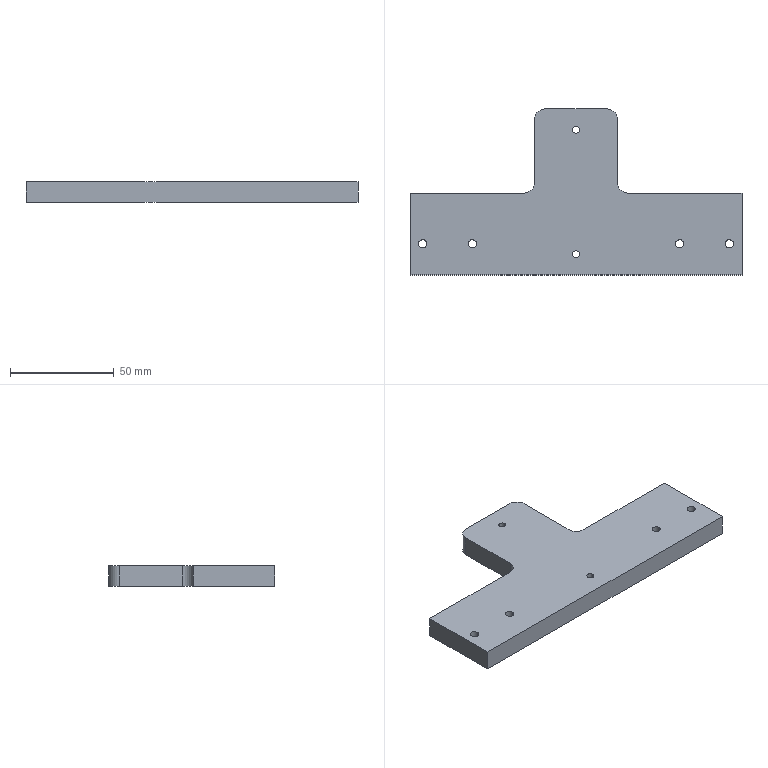Part | 1 solid | 26 faces | box 160 x 80 x 10 mm | volume 78726 mm3 | cylinder 16 | plane 10 | commonest cylinder face diameters 4 x8 3.3 x4 10 x4
STEP:
#1=CARTESIAN_POINT('',(1.65,-30.,0.));
#2=VERTEX_POINT('',#1);
#3=CARTESIAN_POINT('',(-1.65,-30.,0.));
#4=VERTEX_POINT('',#3);
#5=CARTESIAN_POINT('',(0.,-30.,0.));
#6=DIRECTION('',(0.,0.,-1.));
#7=DIRECTION('',(-1.,0.,0.));
#8=AXIS2_PLACEMENT_3D('',#5,#6,#7);
#9=CIRCLE('',#8,1.65);
#10=EDGE_CURVE('',#2,#4,#9,.T.);
#11=ORIENTED_EDGE('',*,*,#10,.T.);
#12=CARTESIAN_POINT('',(-1.65,-30.,10.));
#13=VERTEX_POINT('',#12);
#14=CARTESIAN_POINT('',(-1.65,-30.,10.));
#15=DIRECTION('',(0.,0.,1.));
#16=VECTOR('',#15,1000.);
#17=LINE('',#14,#16);
#18=EDGE_CURVE('',#4,#13,#17,.T.);
#19=ORIENTED_EDGE('',*,*,#18,.T.);
#20=CARTESIAN_POINT('',(1.65,-30.,10.));
#21=VERTEX_POINT('',#20);
#22=CARTESIAN_POINT('',(0.,-30.,10.));
#23=DIRECTION('',(0.,0.,1.));
#24=DIRECTION('',(1.,0.,0.));
#25=AXIS2_PLACEMENT_3D('',#22,#23,#24);
#26=CIRCLE('',#25,1.65);
#27=EDGE_CURVE('',#13,#21,#26,.T.);
#28=ORIENTED_EDGE('',*,*,#27,.T.);
#29=CARTESIAN_POINT('',(1.65,-30.,10.));
#30=DIRECTION('',(0.,0.,1.));
#31=VECTOR('',#30,1000.);
#32=LINE('',#29,#31);
#33=EDGE_CURVE('',#2,#21,#32,.T.);
#34=ORIENTED_EDGE('',*,*,#33,.F.);
#35=EDGE_LOOP('',(#11,#19,#28,#34));
#36=FACE_OUTER_BOUND('',#35,.T.);
#37=CARTESIAN_POINT('',(0.,-30.,10.));
#38=DIRECTION('',(0.,0.,1.));
#39=DIRECTION('',(1.,0.,0.));
#40=AXIS2_PLACEMENT_3D('',#37,#38,#39);
#41=CYLINDRICAL_SURFACE('',#40,1.65);
#42=ADVANCED_FACE('',(#36),#41,.F.);
#43=CARTESIAN_POINT('',(1.65,30.,0.));
#44=VERTEX_POINT('',#43);
#45=CARTESIAN_POINT('',(-1.65,30.,0.));
#46=VERTEX_POINT('',#45);
#47=CARTESIAN_POINT('',(0.,30.,0.));
#48=DIRECTION('',(0.,0.,-1.));
#49=DIRECTION('',(-1.,0.,0.));
#50=AXIS2_PLACEMENT_3D('',#47,#48,#49);
#51=CIRCLE('',#50,1.65);
#52=EDGE_CURVE('',#44,#46,#51,.T.);
#53=ORIENTED_EDGE('',*,*,#52,.T.);
#54=CARTESIAN_POINT('',(-1.65,30.,10.));
#55=VERTEX_POINT('',#54);
#56=CARTESIAN_POINT('',(-1.65,30.,10.));
#57=DIRECTION('',(0.,0.,1.));
#58=VECTOR('',#57,1000.);
#59=LINE('',#56,#58);
#60=EDGE_CURVE('',#46,#55,#59,.T.);
#61=ORIENTED_EDGE('',*,*,#60,.T.);
#62=CARTESIAN_POINT('',(1.65,30.,10.));
#63=VERTEX_POINT('',#62);
#64=CARTESIAN_POINT('',(0.,30.,10.));
#65=DIRECTION('',(0.,0.,1.));
#66=DIRECTION('',(1.,0.,0.));
#67=AXIS2_PLACEMENT_3D('',#64,#65,#66);
#68=CIRCLE('',#67,1.65);
#69=EDGE_CURVE('',#55,#63,#68,.T.);
#70=ORIENTED_EDGE('',*,*,#69,.T.);
#71=CARTESIAN_POINT('',(1.65,30.,10.));
#72=DIRECTION('',(0.,0.,1.));
#73=VECTOR('',#72,1000.);
#74=LINE('',#71,#73);
#75=EDGE_CURVE('',#44,#63,#74,.T.);
#76=ORIENTED_EDGE('',*,*,#75,.F.);
#77=EDGE_LOOP('',(#53,#61,#70,#76));
#78=FACE_OUTER_BOUND('',#77,.T.);
#79=CARTESIAN_POINT('',(0.,30.,10.));
#80=DIRECTION('',(0.,0.,1.));
#81=DIRECTION('',(1.,0.,0.));
#82=AXIS2_PLACEMENT_3D('',#79,#80,#81);
#83=CYLINDRICAL_SURFACE('',#82,1.65);
#84=ADVANCED_FACE('',(#78),#83,.F.);
#85=CARTESIAN_POINT('',(71.9,-25.,10.));
#86=VERTEX_POINT('',#85);
#87=CARTESIAN_POINT('',(75.9,-25.,10.));
#88=VERTEX_POINT('',#87);
#89=CARTESIAN_POINT('',(73.9,-25.,10.));
#90=DIRECTION('',(0.,0.,1.));
#91=DIRECTION('',(1.,0.,0.));
#92=AXIS2_PLACEMENT_3D('',#89,#90,#91);
#93=CIRCLE('',#92,2.);
#94=EDGE_CURVE('',#86,#88,#93,.T.);
#95=ORIENTED_EDGE('',*,*,#94,.T.);
#96=CARTESIAN_POINT('',(75.9,-25.,0.));
#97=VERTEX_POINT('',#96);
#98=CARTESIAN_POINT('',(75.9,-25.,10.));
#99=DIRECTION('',(0.,0.,-1.));
#100=VECTOR('',#99,1000.);
#101=LINE('',#98,#100);
#102=EDGE_CURVE('',#88,#97,#101,.T.);
#103=ORIENTED_EDGE('',*,*,#102,.T.);
#104=CARTESIAN_POINT('',(71.9,-25.,0.));
#105=VERTEX_POINT('',#104);
#106=CARTESIAN_POINT('',(73.9,-25.,0.));
#107=DIRECTION('',(0.,0.,1.));
#108=DIRECTION('',(1.,0.,0.));
#109=AXIS2_PLACEMENT_3D('',#106,#107,#108);
#110=CIRCLE('',#109,2.);
#111=EDGE_CURVE('',#105,#97,#110,.T.);
#112=ORIENTED_EDGE('',*,*,#111,.F.);
#113=CARTESIAN_POINT('',(71.9,-25.,10.));
#114=DIRECTION('',(0.,0.,-1.));
#115=VECTOR('',#114,1000.);
#116=LINE('',#113,#115);
#117=EDGE_CURVE('',#86,#105,#116,.T.);
#118=ORIENTED_EDGE('',*,*,#117,.F.);
#119=EDGE_LOOP('',(#95,#103,#112,#118));
#120=FACE_OUTER_BOUND('',#119,.T.);
#121=CARTESIAN_POINT('',(73.9,-25.,10.));
#122=DIRECTION('',(0.,0.,-1.));
#123=DIRECTION('',(-1.,0.,0.));
#124=AXIS2_PLACEMENT_3D('',#121,#122,#123);
#125=CYLINDRICAL_SURFACE('',#124,2.);
#126=ADVANCED_FACE('',(#120),#125,.F.);
#127=CARTESIAN_POINT('',(-75.9,-25.,10.));
#128=VERTEX_POINT('',#127);
#129=CARTESIAN_POINT('',(-71.9,-25.,10.));
#130=VERTEX_POINT('',#129);
#131=CARTESIAN_POINT('',(-73.9,-25.,10.));
#132=DIRECTION('',(0.,0.,1.));
#133=DIRECTION('',(1.,0.,0.));
#134=AXIS2_PLACEMENT_3D('',#131,#132,#133);
#135=CIRCLE('',#134,2.);
#136=EDGE_CURVE('',#128,#130,#135,.T.);
#137=ORIENTED_EDGE('',*,*,#136,.T.);
#138=CARTESIAN_POINT('',(-71.9,-25.,0.));
#139=VERTEX_POINT('',#138);
#140=CARTESIAN_POINT('',(-71.9,-25.,10.));
#141=DIRECTION('',(0.,0.,-1.));
#142=VECTOR('',#141,1000.);
#143=LINE('',#140,#142);
#144=EDGE_CURVE('',#130,#139,#143,.T.);
#145=ORIENTED_EDGE('',*,*,#144,.T.);
#146=CARTESIAN_POINT('',(-75.9,-25.,0.));
#147=VERTEX_POINT('',#146);
#148=CARTESIAN_POINT('',(-73.9,-25.,0.));
#149=DIRECTION('',(0.,0.,1.));
#150=DIRECTION('',(1.,0.,0.));
#151=AXIS2_PLACEMENT_3D('',#148,#149,#150);
#152=CIRCLE('',#151,2.);
#153=EDGE_CURVE('',#147,#139,#152,.T.);
#154=ORIENTED_EDGE('',*,*,#153,.F.);
#155=CARTESIAN_POINT('',(-75.9,-25.,10.));
#156=DIRECTION('',(0.,0.,-1.));
#157=VECTOR('',#156,1000.);
#158=LINE('',#155,#157);
#159=EDGE_CURVE('',#128,#147,#158,.T.);
#160=ORIENTED_EDGE('',*,*,#159,.F.);
#161=EDGE_LOOP('',(#137,#145,#154,#160));
#162=FACE_OUTER_BOUND('',#161,.T.);
#163=CARTESIAN_POINT('',(-73.9,-25.,10.));
#164=DIRECTION('',(0.,0.,-1.));
#165=DIRECTION('',(-1.,0.,0.));
#166=AXIS2_PLACEMENT_3D('',#163,#164,#165);
#167=CYLINDRICAL_SURFACE('',#166,2.);
#168=ADVANCED_FACE('',(#162),#167,.F.);
#169=CARTESIAN_POINT('',(47.9,-25.,10.));
#170=VERTEX_POINT('',#169);
#171=CARTESIAN_POINT('',(51.9,-25.,10.));
#172=VERTEX_POINT('',#171);
#173=CARTESIAN_POINT('',(49.9,-25.,10.));
#174=DIRECTION('',(0.,0.,1.));
#175=DIRECTION('',(1.,0.,0.));
#176=AXIS2_PLACEMENT_3D('',#173,#174,#175);
#177=CIRCLE('',#176,2.);
#178=EDGE_CURVE('',#170,#172,#177,.T.);
#179=ORIENTED_EDGE('',*,*,#178,.T.);
#180=CARTESIAN_POINT('',(51.9,-25.,0.));
#181=VERTEX_POINT('',#180);
#182=CARTESIAN_POINT('',(51.9,-25.,10.));
#183=DIRECTION('',(0.,0.,-1.));
#184=VECTOR('',#183,1000.);
#185=LINE('',#182,#184);
#186=EDGE_CURVE('',#172,#181,#185,.T.);
#187=ORIENTED_EDGE('',*,*,#186,.T.);
#188=CARTESIAN_POINT('',(47.9,-25.,0.));
#189=VERTEX_POINT('',#188);
#190=CARTESIAN_POINT('',(49.9,-25.,0.));
#191=DIRECTION('',(0.,0.,1.));
#192=DIRECTION('',(1.,0.,0.));
#193=AXIS2_PLACEMENT_3D('',#190,#191,#192);
#194=CIRCLE('',#193,2.);
#195=EDGE_CURVE('',#189,#181,#194,.T.);
#196=ORIENTED_EDGE('',*,*,#195,.F.);
#197=CARTESIAN_POINT('',(47.9,-25.,10.));
#198=DIRECTION('',(0.,0.,-1.));
#199=VECTOR('',#198,1000.);
#200=LINE('',#197,#199);
#201=EDGE_CURVE('',#170,#189,#200,.T.);
#202=ORIENTED_EDGE('',*,*,#201,.F.);
#203=EDGE_LOOP('',(#179,#187,#196,#202));
#204=FACE_OUTER_BOUND('',#203,.T.);
#205=CARTESIAN_POINT('',(49.9,-25.,10.));
#206=DIRECTION('',(0.,0.,-1.));
#207=DIRECTION('',(-1.,0.,0.));
#208=AXIS2_PLACEMENT_3D('',#205,#206,#207);
#209=CYLINDRICAL_SURFACE('',#208,2.);
#210=ADVANCED_FACE('',(#204),#209,.F.);
#211=CARTESIAN_POINT('',(-51.9,-25.,10.));
#212=VERTEX_POINT('',#211);
#213=CARTESIAN_POINT('',(-47.9,-25.,10.));
#214=VERTEX_POINT('',#213);
#215=CARTESIAN_POINT('',(-49.9,-25.,10.));
#216=DIRECTION('',(0.,0.,1.));
#217=DIRECTION('',(1.,0.,0.));
#218=AXIS2_PLACEMENT_3D('',#215,#216,#217);
#219=CIRCLE('',#218,2.);
#220=EDGE_CURVE('',#212,#214,#219,.T.);
#221=ORIENTED_EDGE('',*,*,#220,.T.);
#222=CARTESIAN_POINT('',(-47.9,-25.,0.));
#223=VERTEX_POINT('',#222);
#224=CARTESIAN_POINT('',(-47.9,-25.,10.));
#225=DIRECTION('',(0.,0.,-1.));
#226=VECTOR('',#225,1000.);
#227=LINE('',#224,#226);
#228=EDGE_CURVE('',#214,#223,#227,.T.);
#229=ORIENTED_EDGE('',*,*,#228,.T.);
#230=CARTESIAN_POINT('',(-51.9,-25.,0.));
#231=VERTEX_POINT('',#230);
#232=CARTESIAN_POINT('',(-49.9,-25.,0.));
#233=DIRECTION('',(0.,0.,1.));
#234=DIRECTION('',(1.,0.,0.));
#235=AXIS2_PLACEMENT_3D('',#232,#233,#234);
#236=CIRCLE('',#235,2.);
#237=EDGE_CURVE('',#231,#223,#236,.T.);
#238=ORIENTED_EDGE('',*,*,#237,.F.);
#239=CARTESIAN_POINT('',(-51.9,-25.,10.));
#240=DIRECTION('',(0.,0.,-1.));
#241=VECTOR('',#240,1000.);
#242=LINE('',#239,#241);
#243=EDGE_CURVE('',#212,#231,#242,.T.);
#244=ORIENTED_EDGE('',*,*,#243,.F.);
#245=EDGE_LOOP('',(#221,#229,#238,#244));
#246=FACE_OUTER_BOUND('',#245,.T.);
#247=CARTESIAN_POINT('',(-49.9,-25.,10.));
#248=DIRECTION('',(0.,0.,-1.));
#249=DIRECTION('',(-1.,0.,0.));
#250=AXIS2_PLACEMENT_3D('',#247,#248,#249);
#251=CYLINDRICAL_SURFACE('',#250,2.);
#252=ADVANCED_FACE('',(#246),#251,.F.);
#253=CARTESIAN_POINT('',(0.,-30.,10.));
#254=DIRECTION('',(0.,0.,1.));
#255=DIRECTION('',(1.,0.,0.));
#256=AXIS2_PLACEMENT_3D('',#253,#254,#255);
#257=CIRCLE('',#256,1.65);
#258=EDGE_CURVE('',#21,#13,#257,.T.);
#259=ORIENTED_EDGE('',*,*,#258,.F.);
#260=ORIENTED_EDGE('',*,*,#27,.F.);
#261=EDGE_LOOP('',(#259,#260));
#262=FACE_BOUND('',#261,.T.);
#263=CARTESIAN_POINT('',(20.,4.5,10.));
#264=VERTEX_POINT('',#263);
#265=CARTESIAN_POINT('',(20.,35.,10.));
#266=VERTEX_POINT('',#265);
#267=CARTESIAN_POINT('',(20.,40.,10.));
#268=DIRECTION('',(0.,1.,0.));
#269=VECTOR('',#268,1000.);
#270=LINE('',#267,#269);
#271=EDGE_CURVE('',#264,#266,#270,.T.);
#272=ORIENTED_EDGE('',*,*,#271,.T.);
#273=CARTESIAN_POINT('',(15.,40.,10.));
#274=VERTEX_POINT('',#273);
#275=CARTESIAN_POINT('',(15.,35.,10.));
#276=DIRECTION('',(0.,0.,1.));
#277=DIRECTION('',(-1.,0.,0.));
#278=AXIS2_PLACEMENT_3D('',#275,#276,#277);
#279=CIRCLE('',#278,5.);
#280=EDGE_CURVE('',#266,#274,#279,.T.);
#281=ORIENTED_EDGE('',*,*,#280,.T.);
#282=CARTESIAN_POINT('',(-15.,40.,10.));
#283=VERTEX_POINT('',#282);
#284=CARTESIAN_POINT('',(-80.,40.,10.));
#285=DIRECTION('',(-1.,0.,0.));
#286=VECTOR('',#285,1000.);
#287=LINE('',#284,#286);
#288=EDGE_CURVE('',#274,#283,#287,.T.);
#289=ORIENTED_EDGE('',*,*,#288,.T.);
#290=CARTESIAN_POINT('',(-20.,35.,10.));
#291=VERTEX_POINT('',#290);
#292=CARTESIAN_POINT('',(-15.,35.,10.));
#293=DIRECTION('',(0.,0.,1.));
#294=DIRECTION('',(-1.,0.,0.));
#295=AXIS2_PLACEMENT_3D('',#292,#293,#294);
#296=CIRCLE('',#295,5.);
#297=EDGE_CURVE('',#283,#291,#296,.T.);
#298=ORIENTED_EDGE('',*,*,#297,.T.);
#299=CARTESIAN_POINT('',(-20.,4.5,10.));
#300=VERTEX_POINT('',#299);
#301=CARTESIAN_POINT('',(-20.,40.,10.));
#302=DIRECTION('',(0.,1.,0.));
#303=VECTOR('',#302,1000.);
#304=LINE('',#301,#303);
#305=EDGE_CURVE('',#300,#291,#304,.T.);
#306=ORIENTED_EDGE('',*,*,#305,.F.);
#307=CARTESIAN_POINT('',(-25.,-0.5,10.));
#308=VERTEX_POINT('',#307);
#309=CARTESIAN_POINT('',(-25.,4.5,10.));
#310=DIRECTION('',(0.,0.,-1.));
#311=DIRECTION('',(-1.,0.,0.));
#312=AXIS2_PLACEMENT_3D('',#309,#310,#311);
#313=CIRCLE('',#312,5.);
#314=EDGE_CURVE('',#300,#308,#313,.T.);
#315=ORIENTED_EDGE('',*,*,#314,.T.);
#316=CARTESIAN_POINT('',(-80.,-0.5,10.));
#317=VERTEX_POINT('',#316);
#318=CARTESIAN_POINT('',(-20.,-0.5,10.));
#319=DIRECTION('',(1.,0.,0.));
#320=VECTOR('',#319,1000.);
#321=LINE('',#318,#320);
#322=EDGE_CURVE('',#317,#308,#321,.T.);
#323=ORIENTED_EDGE('',*,*,#322,.F.);
#324=CARTESIAN_POINT('',(-80.,-40.,10.));
#325=VERTEX_POINT('',#324);
#326=CARTESIAN_POINT('',(-80.,-40.,10.));
#327=DIRECTION('',(0.,-1.,0.));
#328=VECTOR('',#327,1000.);
#329=LINE('',#326,#328);
#330=EDGE_CURVE('',#317,#325,#329,.T.);
#331=ORIENTED_EDGE('',*,*,#330,.T.);
#332=CARTESIAN_POINT('',(80.,-40.,10.));
#333=VERTEX_POINT('',#332);
#334=CARTESIAN_POINT('',(-80.,-40.,10.));
#335=DIRECTION('',(1.,0.,0.));
#336=VECTOR('',#335,1000.);
#337=LINE('',#334,#336);
#338=EDGE_CURVE('',#325,#333,#337,.T.);
#339=ORIENTED_EDGE('',*,*,#338,.T.);
#340=CARTESIAN_POINT('',(80.,-0.5,10.));
#341=VERTEX_POINT('',#340);
#342=CARTESIAN_POINT('',(80.,-40.,10.));
#343=DIRECTION('',(0.,1.,0.));
#344=VECTOR('',#343,1000.);
#345=LINE('',#342,#344);
#346=EDGE_CURVE('',#333,#341,#345,.T.);
#347=ORIENTED_EDGE('',*,*,#346,.T.);
#348=CARTESIAN_POINT('',(25.,-0.5,10.));
#349=VERTEX_POINT('',#348);
#350=CARTESIAN_POINT('',(20.,-0.5,10.));
#351=DIRECTION('',(-1.,0.,0.));
#352=VECTOR('',#351,1000.);
#353=LINE('',#350,#352);
#354=EDGE_CURVE('',#341,#349,#353,.T.);
#355=ORIENTED_EDGE('',*,*,#354,.T.);
#356=CARTESIAN_POINT('',(25.,4.5,10.));
#357=DIRECTION('',(0.,0.,-1.));
#358=DIRECTION('',(-1.,0.,0.));
#359=AXIS2_PLACEMENT_3D('',#356,#357,#358);
#360=CIRCLE('',#359,5.);
#361=EDGE_CURVE('',#349,#264,#360,.T.);
#362=ORIENTED_EDGE('',*,*,#361,.T.);
#363=EDGE_LOOP('',(#272,#281,#289,#298,#306,#315,#323,#331,#339,#347,#355,#362));
#364=FACE_OUTER_BOUND('',#363,.T.);
#365=ORIENTED_EDGE('',*,*,#136,.F.);
#366=CARTESIAN_POINT('',(-73.9,-25.,10.));
#367=DIRECTION('',(0.,0.,1.));
#368=DIRECTION('',(1.,0.,0.));
#369=AXIS2_PLACEMENT_3D('',#366,#367,#368);
#370=CIRCLE('',#369,2.);
#371=EDGE_CURVE('',#130,#128,#370,.T.);
#372=ORIENTED_EDGE('',*,*,#371,.F.);
#373=EDGE_LOOP('',(#365,#372));
#374=FACE_BOUND('',#373,.T.);
#375=ORIENTED_EDGE('',*,*,#220,.F.);
#376=CARTESIAN_POINT('',(-49.9,-25.,10.));
#377=DIRECTION('',(0.,0.,1.));
#378=DIRECTION('',(1.,0.,0.));
#379=AXIS2_PLACEMENT_3D('',#376,#377,#378);
#380=CIRCLE('',#379,2.);
#381=EDGE_CURVE('',#214,#212,#380,.T.);
#382=ORIENTED_EDGE('',*,*,#381,.F.);
#383=EDGE_LOOP('',(#375,#382));
#384=FACE_BOUND('',#383,.T.);
#385=ORIENTED_EDGE('',*,*,#178,.F.);
#386=CARTESIAN_POINT('',(49.9,-25.,10.));
#387=DIRECTION('',(0.,0.,1.));
#388=DIRECTION('',(1.,0.,0.));
#389=AXIS2_PLACEMENT_3D('',#386,#387,#388);
#390=CIRCLE('',#389,2.);
#391=EDGE_CURVE('',#172,#170,#390,.T.);
#392=ORIENTED_EDGE('',*,*,#391,.F.);
#393=EDGE_LOOP('',(#385,#392));
#394=FACE_BOUND('',#393,.T.);
#395=ORIENTED_EDGE('',*,*,#94,.F.);
#396=CARTESIAN_POINT('',(73.9,-25.,10.));
#397=DIRECTION('',(0.,0.,1.));
#398=DIRECTION('',(1.,0.,0.));
#399=AXIS2_PLACEMENT_3D('',#396,#397,#398);
#400=CIRCLE('',#399,2.);
#401=EDGE_CURVE('',#88,#86,#400,.T.);
#402=ORIENTED_EDGE('',*,*,#401,.F.);
#403=EDGE_LOOP('',(#395,#402));
#404=FACE_BOUND('',#403,.T.);
#405=CARTESIAN_POINT('',(0.,30.,10.));
#406=DIRECTION('',(0.,0.,1.));
#407=DIRECTION('',(1.,0.,0.));
#408=AXIS2_PLACEMENT_3D('',#405,#406,#407);
#409=CIRCLE('',#408,1.65);
#410=EDGE_CURVE('',#63,#55,#409,.T.);
#411=ORIENTED_EDGE('',*,*,#410,.F.);
#412=ORIENTED_EDGE('',*,*,#69,.F.);
#413=EDGE_LOOP('',(#411,#412));
#414=FACE_BOUND('',#413,.T.);
#415=CARTESIAN_POINT('',(0.,0.,10.));
#416=DIRECTION('',(0.,0.,-1.));
#417=DIRECTION('',(-1.,0.,0.));
#418=AXIS2_PLACEMENT_3D('',#415,#416,#417);
#419=PLANE('',#418);
#420=ADVANCED_FACE('',(#262,#364,#374,#384,#394,#404,#414),#419,.F.);
#421=ORIENTED_EDGE('',*,*,#10,.F.);
#422=CARTESIAN_POINT('',(0.,-30.,0.));
#423=DIRECTION('',(0.,0.,-1.));
#424=DIRECTION('',(-1.,0.,0.));
#425=AXIS2_PLACEMENT_3D('',#422,#423,#424);
#426=CIRCLE('',#425,1.65);
#427=EDGE_CURVE('',#4,#2,#426,.T.);
#428=ORIENTED_EDGE('',*,*,#427,.F.);
#429=EDGE_LOOP('',(#421,#428));
#430=FACE_BOUND('',#429,.T.);
#431=ORIENTED_EDGE('',*,*,#52,.F.);
#432=CARTESIAN_POINT('',(0.,30.,0.));
#433=DIRECTION('',(0.,0.,-1.));
#434=DIRECTION('',(-1.,0.,0.));
#435=AXIS2_PLACEMENT_3D('',#432,#433,#434);
#436=CIRCLE('',#435,1.65);
#437=EDGE_CURVE('',#46,#44,#436,.T.);
#438=ORIENTED_EDGE('',*,*,#437,.F.);
#439=EDGE_LOOP('',(#431,#438));
#440=FACE_BOUND('',#439,.T.);
#441=ORIENTED_EDGE('',*,*,#111,.T.);
#442=CARTESIAN_POINT('',(73.9,-25.,0.));
#443=DIRECTION('',(0.,0.,1.));
#444=DIRECTION('',(1.,0.,0.));
#445=AXIS2_PLACEMENT_3D('',#442,#443,#444);
#446=CIRCLE('',#445,2.);
#447=EDGE_CURVE('',#97,#105,#446,.T.);
#448=ORIENTED_EDGE('',*,*,#447,.T.);
#449=EDGE_LOOP('',(#441,#448));
#450=FACE_BOUND('',#449,.T.);
#451=ORIENTED_EDGE('',*,*,#195,.T.);
#452=CARTESIAN_POINT('',(49.9,-25.,0.));
#453=DIRECTION('',(0.,0.,1.));
#454=DIRECTION('',(1.,0.,0.));
#455=AXIS2_PLACEMENT_3D('',#452,#453,#454);
#456=CIRCLE('',#455,2.);
#457=EDGE_CURVE('',#181,#189,#456,.T.);
#458=ORIENTED_EDGE('',*,*,#457,.T.);
#459=EDGE_LOOP('',(#451,#458));
#460=FACE_BOUND('',#459,.T.);
#461=ORIENTED_EDGE('',*,*,#237,.T.);
#462=CARTESIAN_POINT('',(-49.9,-25.,0.));
#463=DIRECTION('',(0.,0.,1.));
#464=DIRECTION('',(1.,0.,0.));
#465=AXIS2_PLACEMENT_3D('',#462,#463,#464);
#466=CIRCLE('',#465,2.);
#467=EDGE_CURVE('',#223,#231,#466,.T.);
#468=ORIENTED_EDGE('',*,*,#467,.T.);
#469=EDGE_LOOP('',(#461,#468));
#470=FACE_BOUND('',#469,.T.);
#471=ORIENTED_EDGE('',*,*,#153,.T.);
#472=CARTESIAN_POINT('',(-73.9,-25.,0.));
#473=DIRECTION('',(0.,0.,1.));
#474=DIRECTION('',(1.,0.,0.));
#475=AXIS2_PLACEMENT_3D('',#472,#473,#474);
#476=CIRCLE('',#475,2.);
#477=EDGE_CURVE('',#139,#147,#476,.T.);
#478=ORIENTED_EDGE('',*,*,#477,.T.);
#479=EDGE_LOOP('',(#471,#478));
#480=FACE_BOUND('',#479,.T.);
#481=CARTESIAN_POINT('',(15.,40.,0.));
#482=VERTEX_POINT('',#481);
#483=CARTESIAN_POINT('',(-15.,40.,0.));
#484=VERTEX_POINT('',#483);
#485=CARTESIAN_POINT('',(-80.,40.,0.));
#486=DIRECTION('',(-1.,0.,0.));
#487=VECTOR('',#486,1000.);
#488=LINE('',#485,#487);
#489=EDGE_CURVE('',#482,#484,#488,.T.);
#490=ORIENTED_EDGE('',*,*,#489,.F.);
#491=CARTESIAN_POINT('',(20.,35.,0.));
#492=VERTEX_POINT('',#491);
#493=CARTESIAN_POINT('',(15.,35.,0.));
#494=DIRECTION('',(0.,0.,-1.));
#495=DIRECTION('',(-1.,0.,0.));
#496=AXIS2_PLACEMENT_3D('',#493,#494,#495);
#497=CIRCLE('',#496,5.);
#498=EDGE_CURVE('',#482,#492,#497,.T.);
#499=ORIENTED_EDGE('',*,*,#498,.T.);
#500=CARTESIAN_POINT('',(20.,4.5,0.));
#501=VERTEX_POINT('',#500);
#502=CARTESIAN_POINT('',(20.,40.,0.));
#503=DIRECTION('',(0.,1.,0.));
#504=VECTOR('',#503,1000.);
#505=LINE('',#502,#504);
#506=EDGE_CURVE('',#501,#492,#505,.T.);
#507=ORIENTED_EDGE('',*,*,#506,.F.);
#508=CARTESIAN_POINT('',(25.,-0.5,0.));
#509=VERTEX_POINT('',#508);
#510=CARTESIAN_POINT('',(25.,4.5,0.));
#511=DIRECTION('',(0.,0.,1.));
#512=DIRECTION('',(-1.,0.,0.));
#513=AXIS2_PLACEMENT_3D('',#510,#511,#512);
#514=CIRCLE('',#513,5.);
#515=EDGE_CURVE('',#501,#509,#514,.T.);
#516=ORIENTED_EDGE('',*,*,#515,.T.);
#517=CARTESIAN_POINT('',(80.,-0.5,0.));
#518=VERTEX_POINT('',#517);
#519=CARTESIAN_POINT('',(20.,-0.5,0.));
#520=DIRECTION('',(-1.,0.,0.));
#521=VECTOR('',#520,1000.);
#522=LINE('',#519,#521);
#523=EDGE_CURVE('',#518,#509,#522,.T.);
#524=ORIENTED_EDGE('',*,*,#523,.F.);
#525=CARTESIAN_POINT('',(80.,-40.,0.));
#526=VERTEX_POINT('',#525);
#527=CARTESIAN_POINT('',(80.,-40.,0.));
#528=DIRECTION('',(0.,1.,0.));
#529=VECTOR('',#528,1000.);
#530=LINE('',#527,#529);
#531=EDGE_CURVE('',#526,#518,#530,.T.);
#532=ORIENTED_EDGE('',*,*,#531,.F.);
#533=CARTESIAN_POINT('',(-80.,-40.,0.));
#534=VERTEX_POINT('',#533);
#535=CARTESIAN_POINT('',(-80.,-40.,0.));
#536=DIRECTION('',(1.,0.,0.));
#537=VECTOR('',#536,1000.);
#538=LINE('',#535,#537);
#539=EDGE_CURVE('',#534,#526,#538,.T.);
#540=ORIENTED_EDGE('',*,*,#539,.F.);
#541=CARTESIAN_POINT('',(-80.,-0.5,0.));
#542=VERTEX_POINT('',#541);
#543=CARTESIAN_POINT('',(-80.,-40.,0.));
#544=DIRECTION('',(0.,-1.,0.));
#545=VECTOR('',#544,1000.);
#546=LINE('',#543,#545);
#547=EDGE_CURVE('',#542,#534,#546,.T.);
#548=ORIENTED_EDGE('',*,*,#547,.F.);
#549=CARTESIAN_POINT('',(-25.,-0.5,0.));
#550=VERTEX_POINT('',#549);
#551=CARTESIAN_POINT('',(-20.,-0.5,0.));
#552=DIRECTION('',(1.,0.,0.));
#553=VECTOR('',#552,1000.);
#554=LINE('',#551,#553);
#555=EDGE_CURVE('',#542,#550,#554,.T.);
#556=ORIENTED_EDGE('',*,*,#555,.T.);
#557=CARTESIAN_POINT('',(-20.,4.5,0.));
#558=VERTEX_POINT('',#557);
#559=CARTESIAN_POINT('',(-25.,4.5,0.));
#560=DIRECTION('',(0.,0.,1.));
#561=DIRECTION('',(-1.,0.,0.));
#562=AXIS2_PLACEMENT_3D('',#559,#560,#561);
#563=CIRCLE('',#562,5.);
#564=EDGE_CURVE('',#550,#558,#563,.T.);
#565=ORIENTED_EDGE('',*,*,#564,.T.);
#566=CARTESIAN_POINT('',(-20.,35.,0.));
#567=VERTEX_POINT('',#566);
#568=CARTESIAN_POINT('',(-20.,40.,0.));
#569=DIRECTION('',(0.,1.,0.));
#570=VECTOR('',#569,1000.);
#571=LINE('',#568,#570);
#572=EDGE_CURVE('',#558,#567,#571,.T.);
#573=ORIENTED_EDGE('',*,*,#572,.T.);
#574=CARTESIAN_POINT('',(-15.,35.,0.));
#575=DIRECTION('',(0.,0.,-1.));
#576=DIRECTION('',(-1.,0.,0.));
#577=AXIS2_PLACEMENT_3D('',#574,#575,#576);
#578=CIRCLE('',#577,5.);
#579=EDGE_CURVE('',#567,#484,#578,.T.);
#580=ORIENTED_EDGE('',*,*,#579,.T.);
#581=EDGE_LOOP('',(#490,#499,#507,#516,#524,#532,#540,#548,#556,#565,#573,#580));
#582=FACE_OUTER_BOUND('',#581,.T.);
#583=CARTESIAN_POINT('',(0.,0.,0.));
#584=DIRECTION('',(0.,0.,-1.));
#585=DIRECTION('',(-1.,0.,0.));
#586=AXIS2_PLACEMENT_3D('',#583,#584,#585);
#587=PLANE('',#586);
#588=ADVANCED_FACE('',(#430,#440,#450,#460,#470,#480,#582),#587,.T.);
#589=CARTESIAN_POINT('',(80.,-0.5,0.));
#590=DIRECTION('',(0.,0.,1.));
#591=VECTOR('',#590,1000.);
#592=LINE('',#589,#591);
#593=EDGE_CURVE('',#518,#341,#592,.T.);
#594=ORIENTED_EDGE('',*,*,#593,.T.);
#595=ORIENTED_EDGE('',*,*,#346,.F.);
#596=CARTESIAN_POINT('',(80.,-40.,10.));
#597=DIRECTION('',(0.,0.,-1.));
#598=VECTOR('',#597,1000.);
#599=LINE('',#596,#598);
#600=EDGE_CURVE('',#333,#526,#599,.T.);
#601=ORIENTED_EDGE('',*,*,#600,.T.);
#602=ORIENTED_EDGE('',*,*,#531,.T.);
#603=EDGE_LOOP('',(#594,#595,#601,#602));
#604=FACE_OUTER_BOUND('',#603,.T.);
#605=CARTESIAN_POINT('',(80.,-40.,10.));
#606=DIRECTION('',(-1.,0.,0.));
#607=DIRECTION('',(0.,-1.,0.));
#608=AXIS2_PLACEMENT_3D('',#605,#606,#607);
#609=PLANE('',#608);
#610=ADVANCED_FACE('',(#604),#609,.F.);
#611=ORIENTED_EDGE('',*,*,#288,.F.);
#612=CARTESIAN_POINT('',(15.,40.,0.));
#613=DIRECTION('',(0.,0.,-1.));
#614=VECTOR('',#613,1000.);
#615=LINE('',#612,#614);
#616=EDGE_CURVE('',#274,#482,#615,.T.);
#617=ORIENTED_EDGE('',*,*,#616,.T.);
#618=ORIENTED_EDGE('',*,*,#489,.T.);
#619=CARTESIAN_POINT('',(-15.,40.,10.));
#620=DIRECTION('',(0.,0.,1.));
#621=VECTOR('',#620,1000.);
#622=LINE('',#619,#621);
#623=EDGE_CURVE('',#484,#283,#622,.T.);
#624=ORIENTED_EDGE('',*,*,#623,.T.);
#625=EDGE_LOOP('',(#611,#617,#618,#624));
#626=FACE_OUTER_BOUND('',#625,.T.);
#627=CARTESIAN_POINT('',(-80.,40.,10.));
#628=DIRECTION('',(0.,-1.,0.));
#629=DIRECTION('',(1.,0.,0.));
#630=AXIS2_PLACEMENT_3D('',#627,#628,#629);
#631=PLANE('',#630);
#632=ADVANCED_FACE('',(#626),#631,.F.);
#633=ORIENTED_EDGE('',*,*,#330,.F.);
#634=CARTESIAN_POINT('',(-80.,-0.5,0.));
#635=DIRECTION('',(0.,0.,1.));
#636=VECTOR('',#635,1000.);
#637=LINE('',#634,#636);
#638=EDGE_CURVE('',#542,#317,#637,.T.);
#639=ORIENTED_EDGE('',*,*,#638,.F.);
#640=ORIENTED_EDGE('',*,*,#547,.T.);
#641=CARTESIAN_POINT('',(-80.,-40.,10.));
#642=DIRECTION('',(0.,0.,-1.));
#643=VECTOR('',#642,1000.);
#644=LINE('',#641,#643);
#645=EDGE_CURVE('',#325,#534,#644,.T.);
#646=ORIENTED_EDGE('',*,*,#645,.F.);
#647=EDGE_LOOP('',(#633,#639,#640,#646));
#648=FACE_OUTER_BOUND('',#647,.T.);
#649=CARTESIAN_POINT('',(-80.,-40.,10.));
#650=DIRECTION('',(1.,0.,0.));
#651=DIRECTION('',(0.,1.,0.));
#652=AXIS2_PLACEMENT_3D('',#649,#650,#651);
#653=PLANE('',#652);
#654=ADVANCED_FACE('',(#648),#653,.F.);
#655=ORIENTED_EDGE('',*,*,#539,.T.);
#656=ORIENTED_EDGE('',*,*,#600,.F.);
#657=ORIENTED_EDGE('',*,*,#338,.F.);
#658=ORIENTED_EDGE('',*,*,#645,.T.);
#659=EDGE_LOOP('',(#655,#656,#657,#658));
#660=FACE_OUTER_BOUND('',#659,.T.);
#661=CARTESIAN_POINT('',(-80.,-40.,10.));
#662=DIRECTION('',(0.,1.,0.));
#663=DIRECTION('',(-1.,0.,0.));
#664=AXIS2_PLACEMENT_3D('',#661,#662,#663);
#665=PLANE('',#664);
#666=ADVANCED_FACE('',(#660),#665,.F.);
#667=ORIENTED_EDGE('',*,*,#228,.F.);
#668=ORIENTED_EDGE('',*,*,#381,.T.);
#669=ORIENTED_EDGE('',*,*,#243,.T.);
#670=ORIENTED_EDGE('',*,*,#467,.F.);
#671=EDGE_LOOP('',(#667,#668,#669,#670));
#672=FACE_OUTER_BOUND('',#671,.T.);
#673=CARTESIAN_POINT('',(-49.9,-25.,10.));
#674=DIRECTION('',(0.,0.,-1.));
#675=DIRECTION('',(-1.,0.,0.));
#676=AXIS2_PLACEMENT_3D('',#673,#674,#675);
#677=CYLINDRICAL_SURFACE('',#676,2.);
#678=ADVANCED_FACE('',(#672),#677,.F.);
#679=ORIENTED_EDGE('',*,*,#186,.F.);
#680=ORIENTED_EDGE('',*,*,#391,.T.);
#681=ORIENTED_EDGE('',*,*,#201,.T.);
#682=ORIENTED_EDGE('',*,*,#457,.F.);
#683=EDGE_LOOP('',(#679,#680,#681,#682));
#684=FACE_OUTER_BOUND('',#683,.T.);
#685=CARTESIAN_POINT('',(49.9,-25.,10.));
#686=DIRECTION('',(0.,0.,-1.));
#687=DIRECTION('',(-1.,0.,0.));
#688=AXIS2_PLACEMENT_3D('',#685,#686,#687);
#689=CYLINDRICAL_SURFACE('',#688,2.);
#690=ADVANCED_FACE('',(#684),#689,.F.);
#691=ORIENTED_EDGE('',*,*,#144,.F.);
#692=ORIENTED_EDGE('',*,*,#371,.T.);
#693=ORIENTED_EDGE('',*,*,#159,.T.);
#694=ORIENTED_EDGE('',*,*,#477,.F.);
#695=EDGE_LOOP('',(#691,#692,#693,#694));
#696=FACE_OUTER_BOUND('',#695,.T.);
#697=CARTESIAN_POINT('',(-73.9,-25.,10.));
#698=DIRECTION('',(0.,0.,-1.));
#699=DIRECTION('',(-1.,0.,0.));
#700=AXIS2_PLACEMENT_3D('',#697,#698,#699);
#701=CYLINDRICAL_SURFACE('',#700,2.);
#702=ADVANCED_FACE('',(#696),#701,.F.);
#703=ORIENTED_EDGE('',*,*,#102,.F.);
#704=ORIENTED_EDGE('',*,*,#401,.T.);
#705=ORIENTED_EDGE('',*,*,#117,.T.);
#706=ORIENTED_EDGE('',*,*,#447,.F.);
#707=EDGE_LOOP('',(#703,#704,#705,#706));
#708=FACE_OUTER_BOUND('',#707,.T.);
#709=CARTESIAN_POINT('',(73.9,-25.,10.));
#710=DIRECTION('',(0.,0.,-1.));
#711=DIRECTION('',(-1.,0.,0.));
#712=AXIS2_PLACEMENT_3D('',#709,#710,#711);
#713=CYLINDRICAL_SURFACE('',#712,2.);
#714=ADVANCED_FACE('',(#708),#713,.F.);
#715=ORIENTED_EDGE('',*,*,#572,.F.);
#716=CARTESIAN_POINT('',(-20.,4.5,10.));
#717=DIRECTION('',(0.,0.,1.));
#718=VECTOR('',#717,1000.);
#719=LINE('',#716,#718);
#720=EDGE_CURVE('',#558,#300,#719,.T.);
#721=ORIENTED_EDGE('',*,*,#720,.T.);
#722=ORIENTED_EDGE('',*,*,#305,.T.);
#723=CARTESIAN_POINT('',(-20.,35.,0.));
#724=DIRECTION('',(0.,0.,-1.));
#725=VECTOR('',#724,1000.);
#726=LINE('',#723,#725);
#727=EDGE_CURVE('',#291,#567,#726,.T.);
#728=ORIENTED_EDGE('',*,*,#727,.T.);
#729=EDGE_LOOP('',(#715,#721,#722,#728));
#730=FACE_OUTER_BOUND('',#729,.T.);
#731=CARTESIAN_POINT('',(-20.,40.,0.));
#732=DIRECTION('',(1.,0.,0.));
#733=DIRECTION('',(0.,1.,0.));
#734=AXIS2_PLACEMENT_3D('',#731,#732,#733);
#735=PLANE('',#734);
#736=ADVANCED_FACE('',(#730),#735,.F.);
#737=ORIENTED_EDGE('',*,*,#322,.T.);
#738=CARTESIAN_POINT('',(-25.,-0.5,0.));
#739=DIRECTION('',(0.,0.,-1.));
#740=VECTOR('',#739,1000.);
#741=LINE('',#738,#740);
#742=EDGE_CURVE('',#308,#550,#741,.T.);
#743=ORIENTED_EDGE('',*,*,#742,.T.);
#744=ORIENTED_EDGE('',*,*,#555,.F.);
#745=ORIENTED_EDGE('',*,*,#638,.T.);
#746=EDGE_LOOP('',(#737,#743,#744,#745));
#747=FACE_OUTER_BOUND('',#746,.T.);
#748=CARTESIAN_POINT('',(-20.,-0.5,0.));
#749=DIRECTION('',(0.,-1.,0.));
#750=DIRECTION('',(1.,0.,0.));
#751=AXIS2_PLACEMENT_3D('',#748,#749,#750);
#752=PLANE('',#751);
#753=ADVANCED_FACE('',(#747),#752,.F.);
#754=ORIENTED_EDGE('',*,*,#523,.T.);
#755=CARTESIAN_POINT('',(25.,-0.5,10.));
#756=DIRECTION('',(0.,0.,1.));
#757=VECTOR('',#756,1000.);
#758=LINE('',#755,#757);
#759=EDGE_CURVE('',#509,#349,#758,.T.);
#760=ORIENTED_EDGE('',*,*,#759,.T.);
#761=ORIENTED_EDGE('',*,*,#354,.F.);
#762=ORIENTED_EDGE('',*,*,#593,.F.);
#763=EDGE_LOOP('',(#754,#760,#761,#762));
#764=FACE_OUTER_BOUND('',#763,.T.);
#765=CARTESIAN_POINT('',(20.,-0.5,0.));
#766=DIRECTION('',(0.,1.,0.));
#767=DIRECTION('',(-1.,0.,0.));
#768=AXIS2_PLACEMENT_3D('',#765,#766,#767);
#769=PLANE('',#768);
#770=ADVANCED_FACE('',(#764),#769,.T.);
#771=ORIENTED_EDGE('',*,*,#271,.F.);
#772=CARTESIAN_POINT('',(20.,4.5,0.));
#773=DIRECTION('',(0.,0.,-1.));
#774=VECTOR('',#773,1000.);
#775=LINE('',#772,#774);
#776=EDGE_CURVE('',#264,#501,#775,.T.);
#777=ORIENTED_EDGE('',*,*,#776,.T.);
#778=ORIENTED_EDGE('',*,*,#506,.T.);
#779=CARTESIAN_POINT('',(20.,35.,10.));
#780=DIRECTION('',(0.,0.,1.));
#781=VECTOR('',#780,1000.);
#782=LINE('',#779,#781);
#783=EDGE_CURVE('',#492,#266,#782,.T.);
#784=ORIENTED_EDGE('',*,*,#783,.T.);
#785=EDGE_LOOP('',(#771,#777,#778,#784));
#786=FACE_OUTER_BOUND('',#785,.T.);
#787=CARTESIAN_POINT('',(20.,40.,0.));
#788=DIRECTION('',(1.,0.,0.));
#789=DIRECTION('',(0.,1.,0.));
#790=AXIS2_PLACEMENT_3D('',#787,#788,#789);
#791=PLANE('',#790);
#792=ADVANCED_FACE('',(#786),#791,.T.);
#793=ORIENTED_EDGE('',*,*,#515,.F.);
#794=ORIENTED_EDGE('',*,*,#776,.F.);
#795=ORIENTED_EDGE('',*,*,#361,.F.);
#796=ORIENTED_EDGE('',*,*,#759,.F.);
#797=EDGE_LOOP('',(#793,#794,#795,#796));
#798=FACE_OUTER_BOUND('',#797,.T.);
#799=CARTESIAN_POINT('',(25.,4.5,0.));
#800=DIRECTION('',(0.,0.,-1.));
#801=DIRECTION('',(-1.,0.,0.));
#802=AXIS2_PLACEMENT_3D('',#799,#800,#801);
#803=CYLINDRICAL_SURFACE('',#802,5.);
#804=ADVANCED_FACE('',(#798),#803,.F.);
#805=ORIENTED_EDGE('',*,*,#498,.F.);
#806=ORIENTED_EDGE('',*,*,#616,.F.);
#807=ORIENTED_EDGE('',*,*,#280,.F.);
#808=ORIENTED_EDGE('',*,*,#783,.F.);
#809=EDGE_LOOP('',(#805,#806,#807,#808));
#810=FACE_OUTER_BOUND('',#809,.T.);
#811=CARTESIAN_POINT('',(15.,35.,0.));
#812=DIRECTION('',(0.,0.,-1.));
#813=DIRECTION('',(-1.,0.,0.));
#814=AXIS2_PLACEMENT_3D('',#811,#812,#813);
#815=CYLINDRICAL_SURFACE('',#814,5.);
#816=ADVANCED_FACE('',(#810),#815,.T.);
#817=ORIENTED_EDGE('',*,*,#564,.F.);
#818=ORIENTED_EDGE('',*,*,#742,.F.);
#819=ORIENTED_EDGE('',*,*,#314,.F.);
#820=ORIENTED_EDGE('',*,*,#720,.F.);
#821=EDGE_LOOP('',(#817,#818,#819,#820));
#822=FACE_OUTER_BOUND('',#821,.T.);
#823=CARTESIAN_POINT('',(-25.,4.5,0.));
#824=DIRECTION('',(0.,0.,-1.));
#825=DIRECTION('',(-1.,0.,0.));
#826=AXIS2_PLACEMENT_3D('',#823,#824,#825);
#827=CYLINDRICAL_SURFACE('',#826,5.);
#828=ADVANCED_FACE('',(#822),#827,.F.);
#829=ORIENTED_EDGE('',*,*,#579,.F.);
#830=ORIENTED_EDGE('',*,*,#727,.F.);
#831=ORIENTED_EDGE('',*,*,#297,.F.);
#832=ORIENTED_EDGE('',*,*,#623,.F.);
#833=EDGE_LOOP('',(#829,#830,#831,#832));
#834=FACE_OUTER_BOUND('',#833,.T.);
#835=CARTESIAN_POINT('',(-15.,35.,10.));
#836=DIRECTION('',(0.,0.,1.));
#837=DIRECTION('',(1.,0.,0.));
#838=AXIS2_PLACEMENT_3D('',#835,#836,#837);
#839=CYLINDRICAL_SURFACE('',#838,5.);
#840=ADVANCED_FACE('',(#834),#839,.T.);
#841=ORIENTED_EDGE('',*,*,#60,.F.);
#842=ORIENTED_EDGE('',*,*,#437,.T.);
#843=ORIENTED_EDGE('',*,*,#75,.T.);
#844=ORIENTED_EDGE('',*,*,#410,.T.);
#845=EDGE_LOOP('',(#841,#842,#843,#844));
#846=FACE_OUTER_BOUND('',#845,.T.);
#847=CARTESIAN_POINT('',(0.,30.,10.));
#848=DIRECTION('',(0.,0.,1.));
#849=DIRECTION('',(1.,0.,0.));
#850=AXIS2_PLACEMENT_3D('',#847,#848,#849);
#851=CYLINDRICAL_SURFACE('',#850,1.65);
#852=ADVANCED_FACE('',(#846),#851,.F.);
#853=ORIENTED_EDGE('',*,*,#18,.F.);
#854=ORIENTED_EDGE('',*,*,#427,.T.);
#855=ORIENTED_EDGE('',*,*,#33,.T.);
#856=ORIENTED_EDGE('',*,*,#258,.T.);
#857=EDGE_LOOP('',(#853,#854,#855,#856));
#858=FACE_OUTER_BOUND('',#857,.T.);
#859=CARTESIAN_POINT('',(0.,-30.,10.));
#860=DIRECTION('',(0.,0.,1.));
#861=DIRECTION('',(1.,0.,0.));
#862=AXIS2_PLACEMENT_3D('',#859,#860,#861);
#863=CYLINDRICAL_SURFACE('',#862,1.65);
#864=ADVANCED_FACE('',(#858),#863,.F.);
#865=CLOSED_SHELL('',(#42,#84,#126,#168,#210,#252,#420,#588,#610,#632,#654,#666,#678,#690,#702,#714,#736,#753,#770,#792,#804,#816,#828,#840,#852,#864));
#866=MANIFOLD_SOLID_BREP('',#865);
#867=CARTESIAN_POINT('',(0.,0.,0.));
#868=DIRECTION('',(0.,0.,1.));
#869=DIRECTION('',(1.,0.,0.));
#870=AXIS2_PLACEMENT_3D('',#867,#868,#869);
#871=(LENGTH_UNIT()NAMED_UNIT(*)SI_UNIT(.MILLI.,.METRE.));
#872=UNCERTAINTY_MEASURE_WITH_UNIT(LENGTH_MEASURE(0.00001),#871,'','');
#873=(NAMED_UNIT(*)PLANE_ANGLE_UNIT()SI_UNIT($,.RADIAN.));
#874=(NAMED_UNIT(*)SI_UNIT($,.STERADIAN.)SOLID_ANGLE_UNIT());
#875=(GEOMETRIC_REPRESENTATION_CONTEXT(3)GLOBAL_UNCERTAINTY_ASSIGNED_CONTEXT((#872))GLOBAL_UNIT_ASSIGNED_CONTEXT((#871,#873,#874))REPRESENTATION_CONTEXT('',''));
#876=ADVANCED_BREP_SHAPE_REPRESENTATION('',(#866,#870),#875);